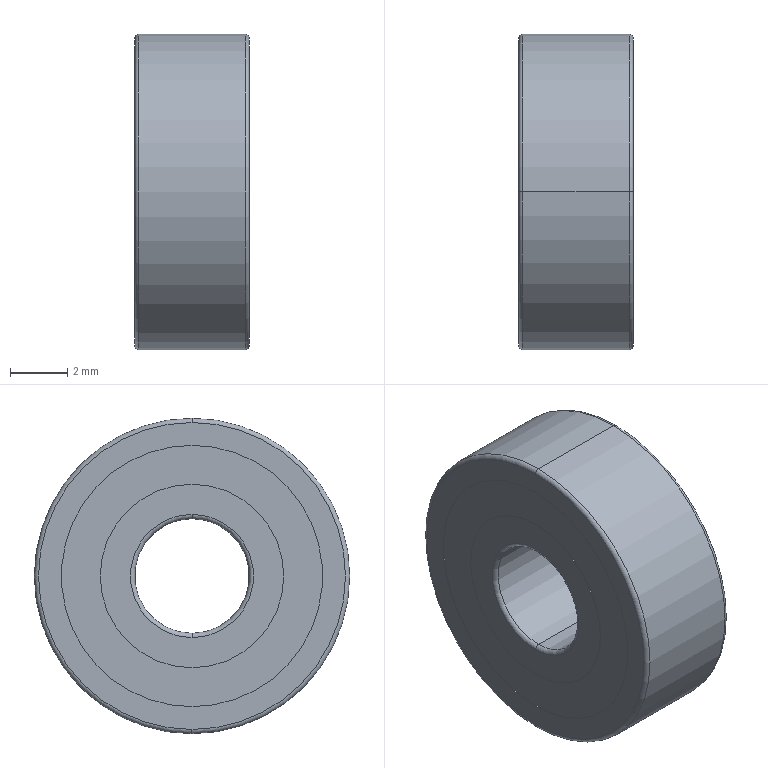Part | SolidWorks | features RefAxis 6, 3DProfileFeature 2, Revolution 1 | 1 solid | 26 faces | box 4 x 11 x 11 mm | volume 327.696 mm3 | cylinder 12 | torus 8 | plane 6 | commonest cylinder face diameters 6.4 x4 9.11 x4 4 x2 11 x2
STEP:
#1=CARTESIAN_POINT('',(3.85,0.,5.5));
#2=VERTEX_POINT('',#1);
#3=CARTESIAN_POINT('',(3.85,0.,-5.5));
#4=VERTEX_POINT('',#3);
#5=CARTESIAN_POINT('',(3.85,0.,0.));
#6=DIRECTION('',(-1.,0.,0.));
#7=DIRECTION('',(0.,0.,1.));
#8=AXIS2_PLACEMENT_3D('',#5,#6,#7);
#9=CIRCLE('',#8,5.5);
#10=EDGE_CURVE('',#2,#4,#9,.T.);
#11=ORIENTED_EDGE('',*,*,#10,.T.);
#12=CARTESIAN_POINT('',(0.15,0.,-5.5));
#13=VERTEX_POINT('',#12);
#14=CARTESIAN_POINT('',(3.85,0.,-5.5));
#15=DIRECTION('',(-1.,0.,0.));
#16=VECTOR('',#15,1000.);
#17=LINE('',#14,#16);
#18=EDGE_CURVE('',#4,#13,#17,.T.);
#19=ORIENTED_EDGE('',*,*,#18,.T.);
#20=CARTESIAN_POINT('',(0.15,0.,5.5));
#21=VERTEX_POINT('',#20);
#22=CARTESIAN_POINT('',(0.15,0.,0.));
#23=DIRECTION('',(-1.,0.,0.));
#24=DIRECTION('',(0.,0.,1.));
#25=AXIS2_PLACEMENT_3D('',#22,#23,#24);
#26=CIRCLE('',#25,5.5);
#27=EDGE_CURVE('',#21,#13,#26,.T.);
#28=ORIENTED_EDGE('',*,*,#27,.F.);
#29=CARTESIAN_POINT('',(3.85,0.,5.5));
#30=DIRECTION('',(-1.,0.,0.));
#31=VECTOR('',#30,1000.);
#32=LINE('',#29,#31);
#33=EDGE_CURVE('',#2,#21,#32,.T.);
#34=ORIENTED_EDGE('',*,*,#33,.F.);
#35=EDGE_LOOP('',(#11,#19,#28,#34));
#36=FACE_OUTER_BOUND('',#35,.T.);
#37=CARTESIAN_POINT('',(3.85,0.,0.));
#38=DIRECTION('',(-1.,0.,0.));
#39=DIRECTION('',(0.,0.,1.));
#40=AXIS2_PLACEMENT_3D('',#37,#38,#39);
#41=CYLINDRICAL_SURFACE('',#40,5.5);
#42=ADVANCED_FACE('',(#36),#41,.T.);
#43=CARTESIAN_POINT('',(4.,0.,5.35));
#44=VERTEX_POINT('',#43);
#45=CARTESIAN_POINT('',(4.,0.,-5.35));
#46=VERTEX_POINT('',#45);
#47=CARTESIAN_POINT('',(4.,0.,0.));
#48=DIRECTION('',(-1.,0.,0.));
#49=DIRECTION('',(0.,0.,1.));
#50=AXIS2_PLACEMENT_3D('',#47,#48,#49);
#51=CIRCLE('',#50,5.35);
#52=EDGE_CURVE('',#44,#46,#51,.T.);
#53=ORIENTED_EDGE('',*,*,#52,.T.);
#54=CARTESIAN_POINT('',(3.85,0.,-5.35));
#55=DIRECTION('',(0.,1.,0.));
#56=DIRECTION('',(0.,0.,1.));
#57=AXIS2_PLACEMENT_3D('',#54,#55,#56);
#58=CIRCLE('',#57,0.15);
#59=EDGE_CURVE('',#46,#4,#58,.T.);
#60=ORIENTED_EDGE('',*,*,#59,.T.);
#61=ORIENTED_EDGE('',*,*,#10,.F.);
#62=CARTESIAN_POINT('',(3.85,0.,5.35));
#63=DIRECTION('',(0.,-1.,0.));
#64=DIRECTION('',(0.,0.,-1.));
#65=AXIS2_PLACEMENT_3D('',#62,#63,#64);
#66=CIRCLE('',#65,0.15);
#67=EDGE_CURVE('',#44,#2,#66,.T.);
#68=ORIENTED_EDGE('',*,*,#67,.F.);
#69=EDGE_LOOP('',(#53,#60,#61,#68));
#70=FACE_OUTER_BOUND('',#69,.T.);
#71=CARTESIAN_POINT('',(3.85,0.,0.));
#72=DIRECTION('',(-1.,0.,0.));
#73=DIRECTION('',(0.,0.,1.));
#74=AXIS2_PLACEMENT_3D('',#71,#72,#73);
#75=TOROIDAL_SURFACE('',#74,5.35,0.15);
#76=ADVANCED_FACE('',(#70),#75,.T.);
#77=CARTESIAN_POINT('',(4.,0.,-4.555));
#78=VERTEX_POINT('',#77);
#79=CARTESIAN_POINT('',(4.,0.,4.555));
#80=VERTEX_POINT('',#79);
#81=CARTESIAN_POINT('',(4.,0.,0.));
#82=DIRECTION('',(-1.,0.,0.));
#83=DIRECTION('',(0.,0.,1.));
#84=AXIS2_PLACEMENT_3D('',#81,#82,#83);
#85=CIRCLE('',#84,4.555);
#86=EDGE_CURVE('',#78,#80,#85,.T.);
#87=ORIENTED_EDGE('',*,*,#86,.F.);
#88=CARTESIAN_POINT('',(3.974,0.,-4.555));
#89=VERTEX_POINT('',#88);
#90=CARTESIAN_POINT('',(3.85,0.,-4.555));
#91=DIRECTION('',(-1.,0.,0.));
#92=VECTOR('',#91,1000.);
#93=LINE('',#90,#92);
#94=EDGE_CURVE('',#78,#89,#93,.T.);
#95=ORIENTED_EDGE('',*,*,#94,.T.);
#96=CARTESIAN_POINT('',(3.974,0.,4.555));
#97=VERTEX_POINT('',#96);
#98=CARTESIAN_POINT('',(3.974,0.,0.));
#99=DIRECTION('',(-1.,0.,0.));
#100=DIRECTION('',(0.,0.,1.));
#101=AXIS2_PLACEMENT_3D('',#98,#99,#100);
#102=CIRCLE('',#101,4.555);
#103=EDGE_CURVE('',#89,#97,#102,.T.);
#104=ORIENTED_EDGE('',*,*,#103,.T.);
#105=CARTESIAN_POINT('',(3.85,0.,4.555));
#106=DIRECTION('',(-1.,0.,0.));
#107=VECTOR('',#106,1000.);
#108=LINE('',#105,#107);
#109=EDGE_CURVE('',#80,#97,#108,.T.);
#110=ORIENTED_EDGE('',*,*,#109,.F.);
#111=EDGE_LOOP('',(#87,#95,#104,#110));
#112=FACE_OUTER_BOUND('',#111,.T.);
#113=CARTESIAN_POINT('',(3.85,0.,0.));
#114=DIRECTION('',(-1.,0.,0.));
#115=DIRECTION('',(0.,0.,1.));
#116=AXIS2_PLACEMENT_3D('',#113,#114,#115);
#117=CYLINDRICAL_SURFACE('',#116,4.555);
#118=ADVANCED_FACE('',(#112),#117,.F.);
#119=CARTESIAN_POINT('',(4.,0.,3.2));
#120=VERTEX_POINT('',#119);
#121=CARTESIAN_POINT('',(4.,0.,-3.2));
#122=VERTEX_POINT('',#121);
#123=CARTESIAN_POINT('',(4.,0.,0.));
#124=DIRECTION('',(-1.,0.,0.));
#125=DIRECTION('',(0.,0.,1.));
#126=AXIS2_PLACEMENT_3D('',#123,#124,#125);
#127=CIRCLE('',#126,3.2);
#128=EDGE_CURVE('',#120,#122,#127,.T.);
#129=ORIENTED_EDGE('',*,*,#128,.T.);
#130=CARTESIAN_POINT('',(3.974,0.,-3.2));
#131=VERTEX_POINT('',#130);
#132=CARTESIAN_POINT('',(3.85,0.,-3.2));
#133=DIRECTION('',(-1.,0.,0.));
#134=VECTOR('',#133,1000.);
#135=LINE('',#132,#134);
#136=EDGE_CURVE('',#122,#131,#135,.T.);
#137=ORIENTED_EDGE('',*,*,#136,.T.);
#138=CARTESIAN_POINT('',(3.974,0.,3.2));
#139=VERTEX_POINT('',#138);
#140=CARTESIAN_POINT('',(3.974,0.,0.));
#141=DIRECTION('',(-1.,0.,0.));
#142=DIRECTION('',(0.,0.,1.));
#143=AXIS2_PLACEMENT_3D('',#140,#141,#142);
#144=CIRCLE('',#143,3.2);
#145=EDGE_CURVE('',#139,#131,#144,.T.);
#146=ORIENTED_EDGE('',*,*,#145,.F.);
#147=CARTESIAN_POINT('',(3.85,0.,3.2));
#148=DIRECTION('',(-1.,0.,0.));
#149=VECTOR('',#148,1000.);
#150=LINE('',#147,#149);
#151=EDGE_CURVE('',#120,#139,#150,.T.);
#152=ORIENTED_EDGE('',*,*,#151,.F.);
#153=EDGE_LOOP('',(#129,#137,#146,#152));
#154=FACE_OUTER_BOUND('',#153,.T.);
#155=CARTESIAN_POINT('',(3.85,0.,0.));
#156=DIRECTION('',(-1.,0.,0.));
#157=DIRECTION('',(0.,0.,1.));
#158=AXIS2_PLACEMENT_3D('',#155,#156,#157);
#159=CYLINDRICAL_SURFACE('',#158,3.2);
#160=ADVANCED_FACE('',(#154),#159,.T.);
#161=CARTESIAN_POINT('',(3.85,0.,2.));
#162=VERTEX_POINT('',#161);
#163=CARTESIAN_POINT('',(3.85,0.,-2.));
#164=VERTEX_POINT('',#163);
#165=CARTESIAN_POINT('',(3.85,0.,0.));
#166=DIRECTION('',(-1.,0.,0.));
#167=DIRECTION('',(0.,0.,1.));
#168=AXIS2_PLACEMENT_3D('',#165,#166,#167);
#169=CIRCLE('',#168,2.);
#170=EDGE_CURVE('',#162,#164,#169,.T.);
#171=ORIENTED_EDGE('',*,*,#170,.T.);
#172=CARTESIAN_POINT('',(4.,0.,-2.15));
#173=VERTEX_POINT('',#172);
#174=CARTESIAN_POINT('',(3.85,0.,-2.15));
#175=DIRECTION('',(0.,1.,0.));
#176=DIRECTION('',(0.,0.,1.));
#177=AXIS2_PLACEMENT_3D('',#174,#175,#176);
#178=CIRCLE('',#177,0.15);
#179=EDGE_CURVE('',#164,#173,#178,.T.);
#180=ORIENTED_EDGE('',*,*,#179,.T.);
#181=CARTESIAN_POINT('',(4.,0.,2.15));
#182=VERTEX_POINT('',#181);
#183=CARTESIAN_POINT('',(4.,0.,0.));
#184=DIRECTION('',(-1.,0.,0.));
#185=DIRECTION('',(0.,0.,1.));
#186=AXIS2_PLACEMENT_3D('',#183,#184,#185);
#187=CIRCLE('',#186,2.15);
#188=EDGE_CURVE('',#182,#173,#187,.T.);
#189=ORIENTED_EDGE('',*,*,#188,.F.);
#190=CARTESIAN_POINT('',(3.85,0.,2.15));
#191=DIRECTION('',(0.,-1.,0.));
#192=DIRECTION('',(0.,0.,-1.));
#193=AXIS2_PLACEMENT_3D('',#190,#191,#192);
#194=CIRCLE('',#193,0.15);
#195=EDGE_CURVE('',#162,#182,#194,.T.);
#196=ORIENTED_EDGE('',*,*,#195,.F.);
#197=EDGE_LOOP('',(#171,#180,#189,#196));
#198=FACE_OUTER_BOUND('',#197,.T.);
#199=CARTESIAN_POINT('',(3.85,0.,0.));
#200=DIRECTION('',(-1.,0.,0.));
#201=DIRECTION('',(0.,0.,1.));
#202=AXIS2_PLACEMENT_3D('',#199,#200,#201);
#203=TOROIDAL_SURFACE('',#202,2.15,0.15);
#204=ADVANCED_FACE('',(#198),#203,.T.);
#205=CARTESIAN_POINT('',(3.85,0.,0.));
#206=DIRECTION('',(-1.,0.,0.));
#207=DIRECTION('',(0.,0.,1.));
#208=AXIS2_PLACEMENT_3D('',#205,#206,#207);
#209=CIRCLE('',#208,2.);
#210=EDGE_CURVE('',#164,#162,#209,.T.);
#211=ORIENTED_EDGE('',*,*,#210,.F.);
#212=CARTESIAN_POINT('',(0.15,0.,-2.));
#213=VERTEX_POINT('',#212);
#214=CARTESIAN_POINT('',(3.85,0.,-2.));
#215=DIRECTION('',(-1.,0.,0.));
#216=VECTOR('',#215,1000.);
#217=LINE('',#214,#216);
#218=EDGE_CURVE('',#164,#213,#217,.T.);
#219=ORIENTED_EDGE('',*,*,#218,.T.);
#220=CARTESIAN_POINT('',(0.15,0.,2.));
#221=VERTEX_POINT('',#220);
#222=CARTESIAN_POINT('',(0.15,0.,0.));
#223=DIRECTION('',(-1.,0.,0.));
#224=DIRECTION('',(0.,0.,1.));
#225=AXIS2_PLACEMENT_3D('',#222,#223,#224);
#226=CIRCLE('',#225,2.);
#227=EDGE_CURVE('',#213,#221,#226,.T.);
#228=ORIENTED_EDGE('',*,*,#227,.T.);
#229=CARTESIAN_POINT('',(3.85,0.,2.));
#230=DIRECTION('',(-1.,0.,0.));
#231=VECTOR('',#230,1000.);
#232=LINE('',#229,#231);
#233=EDGE_CURVE('',#162,#221,#232,.T.);
#234=ORIENTED_EDGE('',*,*,#233,.F.);
#235=EDGE_LOOP('',(#211,#219,#228,#234));
#236=FACE_OUTER_BOUND('',#235,.T.);
#237=CARTESIAN_POINT('',(3.85,0.,0.));
#238=DIRECTION('',(-1.,0.,0.));
#239=DIRECTION('',(0.,0.,1.));
#240=AXIS2_PLACEMENT_3D('',#237,#238,#239);
#241=CYLINDRICAL_SURFACE('',#240,2.);
#242=ADVANCED_FACE('',(#236),#241,.F.);
#243=CARTESIAN_POINT('',(0.,0.,2.15));
#244=VERTEX_POINT('',#243);
#245=CARTESIAN_POINT('',(0.,0.,-2.15));
#246=VERTEX_POINT('',#245);
#247=CARTESIAN_POINT('',(0.,0.,0.));
#248=DIRECTION('',(-1.,0.,0.));
#249=DIRECTION('',(0.,0.,1.));
#250=AXIS2_PLACEMENT_3D('',#247,#248,#249);
#251=CIRCLE('',#250,2.15);
#252=EDGE_CURVE('',#244,#246,#251,.T.);
#253=ORIENTED_EDGE('',*,*,#252,.T.);
#254=CARTESIAN_POINT('',(0.15,0.,-2.15));
#255=DIRECTION('',(0.,1.,0.));
#256=DIRECTION('',(0.,0.,1.));
#257=AXIS2_PLACEMENT_3D('',#254,#255,#256);
#258=CIRCLE('',#257,0.15);
#259=EDGE_CURVE('',#246,#213,#258,.T.);
#260=ORIENTED_EDGE('',*,*,#259,.T.);
#261=CARTESIAN_POINT('',(0.15,0.,0.));
#262=DIRECTION('',(-1.,0.,0.));
#263=DIRECTION('',(0.,0.,1.));
#264=AXIS2_PLACEMENT_3D('',#261,#262,#263);
#265=CIRCLE('',#264,2.);
#266=EDGE_CURVE('',#221,#213,#265,.T.);
#267=ORIENTED_EDGE('',*,*,#266,.F.);
#268=CARTESIAN_POINT('',(0.15,0.,2.15));
#269=DIRECTION('',(0.,-1.,0.));
#270=DIRECTION('',(0.,0.,-1.));
#271=AXIS2_PLACEMENT_3D('',#268,#269,#270);
#272=CIRCLE('',#271,0.15);
#273=EDGE_CURVE('',#244,#221,#272,.T.);
#274=ORIENTED_EDGE('',*,*,#273,.F.);
#275=EDGE_LOOP('',(#253,#260,#267,#274));
#276=FACE_OUTER_BOUND('',#275,.T.);
#277=CARTESIAN_POINT('',(0.15,0.,0.));
#278=DIRECTION('',(-1.,0.,0.));
#279=DIRECTION('',(0.,0.,1.));
#280=AXIS2_PLACEMENT_3D('',#277,#278,#279);
#281=TOROIDAL_SURFACE('',#280,2.15,0.15);
#282=ADVANCED_FACE('',(#276),#281,.T.);
#283=CARTESIAN_POINT('',(0.026,0.,3.2));
#284=VERTEX_POINT('',#283);
#285=CARTESIAN_POINT('',(0.026,0.,-3.2));
#286=VERTEX_POINT('',#285);
#287=CARTESIAN_POINT('',(0.026,0.,0.));
#288=DIRECTION('',(-1.,0.,0.));
#289=DIRECTION('',(0.,0.,1.));
#290=AXIS2_PLACEMENT_3D('',#287,#288,#289);
#291=CIRCLE('',#290,3.2);
#292=EDGE_CURVE('',#284,#286,#291,.T.);
#293=ORIENTED_EDGE('',*,*,#292,.T.);
#294=CARTESIAN_POINT('',(0.,0.,-3.2));
#295=VERTEX_POINT('',#294);
#296=CARTESIAN_POINT('',(3.85,0.,-3.2));
#297=DIRECTION('',(-1.,0.,0.));
#298=VECTOR('',#297,1000.);
#299=LINE('',#296,#298);
#300=EDGE_CURVE('',#286,#295,#299,.T.);
#301=ORIENTED_EDGE('',*,*,#300,.T.);
#302=CARTESIAN_POINT('',(0.,0.,3.2));
#303=VERTEX_POINT('',#302);
#304=CARTESIAN_POINT('',(0.,0.,0.));
#305=DIRECTION('',(-1.,0.,0.));
#306=DIRECTION('',(0.,0.,1.));
#307=AXIS2_PLACEMENT_3D('',#304,#305,#306);
#308=CIRCLE('',#307,3.2);
#309=EDGE_CURVE('',#303,#295,#308,.T.);
#310=ORIENTED_EDGE('',*,*,#309,.F.);
#311=CARTESIAN_POINT('',(3.85,0.,3.2));
#312=DIRECTION('',(-1.,0.,0.));
#313=VECTOR('',#312,1000.);
#314=LINE('',#311,#313);
#315=EDGE_CURVE('',#284,#303,#314,.T.);
#316=ORIENTED_EDGE('',*,*,#315,.F.);
#317=EDGE_LOOP('',(#293,#301,#310,#316));
#318=FACE_OUTER_BOUND('',#317,.T.);
#319=CARTESIAN_POINT('',(3.85,0.,0.));
#320=DIRECTION('',(-1.,0.,0.));
#321=DIRECTION('',(0.,0.,1.));
#322=AXIS2_PLACEMENT_3D('',#319,#320,#321);
#323=CYLINDRICAL_SURFACE('',#322,3.2);
#324=ADVANCED_FACE('',(#318),#323,.T.);
#325=CARTESIAN_POINT('',(0.026,0.,-4.555));
#326=VERTEX_POINT('',#325);
#327=CARTESIAN_POINT('',(0.026,0.,4.555));
#328=VERTEX_POINT('',#327);
#329=CARTESIAN_POINT('',(0.026,0.,0.));
#330=DIRECTION('',(-1.,0.,0.));
#331=DIRECTION('',(0.,0.,1.));
#332=AXIS2_PLACEMENT_3D('',#329,#330,#331);
#333=CIRCLE('',#332,4.555);
#334=EDGE_CURVE('',#326,#328,#333,.T.);
#335=ORIENTED_EDGE('',*,*,#334,.F.);
#336=CARTESIAN_POINT('',(0.,0.,-4.555));
#337=VERTEX_POINT('',#336);
#338=CARTESIAN_POINT('',(3.85,0.,-4.555));
#339=DIRECTION('',(-1.,0.,0.));
#340=VECTOR('',#339,1000.);
#341=LINE('',#338,#340);
#342=EDGE_CURVE('',#326,#337,#341,.T.);
#343=ORIENTED_EDGE('',*,*,#342,.T.);
#344=CARTESIAN_POINT('',(0.,0.,4.555));
#345=VERTEX_POINT('',#344);
#346=CARTESIAN_POINT('',(0.,0.,0.));
#347=DIRECTION('',(-1.,0.,0.));
#348=DIRECTION('',(0.,0.,1.));
#349=AXIS2_PLACEMENT_3D('',#346,#347,#348);
#350=CIRCLE('',#349,4.555);
#351=EDGE_CURVE('',#337,#345,#350,.T.);
#352=ORIENTED_EDGE('',*,*,#351,.T.);
#353=CARTESIAN_POINT('',(3.85,0.,4.555));
#354=DIRECTION('',(-1.,0.,0.));
#355=VECTOR('',#354,1000.);
#356=LINE('',#353,#355);
#357=EDGE_CURVE('',#328,#345,#356,.T.);
#358=ORIENTED_EDGE('',*,*,#357,.F.);
#359=EDGE_LOOP('',(#335,#343,#352,#358));
#360=FACE_OUTER_BOUND('',#359,.T.);
#361=CARTESIAN_POINT('',(3.85,0.,0.));
#362=DIRECTION('',(-1.,0.,0.));
#363=DIRECTION('',(0.,0.,1.));
#364=AXIS2_PLACEMENT_3D('',#361,#362,#363);
#365=CYLINDRICAL_SURFACE('',#364,4.555);
#366=ADVANCED_FACE('',(#360),#365,.F.);
#367=ORIENTED_EDGE('',*,*,#27,.T.);
#368=CARTESIAN_POINT('',(0.,0.,-5.35));
#369=VERTEX_POINT('',#368);
#370=CARTESIAN_POINT('',(0.15,0.,-5.35));
#371=DIRECTION('',(0.,1.,0.));
#372=DIRECTION('',(0.,0.,1.));
#373=AXIS2_PLACEMENT_3D('',#370,#371,#372);
#374=CIRCLE('',#373,0.15);
#375=EDGE_CURVE('',#13,#369,#374,.T.);
#376=ORIENTED_EDGE('',*,*,#375,.T.);
#377=CARTESIAN_POINT('',(0.,0.,5.35));
#378=VERTEX_POINT('',#377);
#379=CARTESIAN_POINT('',(0.,0.,0.));
#380=DIRECTION('',(-1.,0.,0.));
#381=DIRECTION('',(0.,0.,1.));
#382=AXIS2_PLACEMENT_3D('',#379,#380,#381);
#383=CIRCLE('',#382,5.35);
#384=EDGE_CURVE('',#378,#369,#383,.T.);
#385=ORIENTED_EDGE('',*,*,#384,.F.);
#386=CARTESIAN_POINT('',(0.15,0.,5.35));
#387=DIRECTION('',(0.,-1.,0.));
#388=DIRECTION('',(0.,0.,-1.));
#389=AXIS2_PLACEMENT_3D('',#386,#387,#388);
#390=CIRCLE('',#389,0.15);
#391=EDGE_CURVE('',#21,#378,#390,.T.);
#392=ORIENTED_EDGE('',*,*,#391,.F.);
#393=EDGE_LOOP('',(#367,#376,#385,#392));
#394=FACE_OUTER_BOUND('',#393,.T.);
#395=CARTESIAN_POINT('',(0.15,0.,0.));
#396=DIRECTION('',(-1.,0.,0.));
#397=DIRECTION('',(0.,0.,1.));
#398=AXIS2_PLACEMENT_3D('',#395,#396,#397);
#399=TOROIDAL_SURFACE('',#398,5.35,0.15);
#400=ADVANCED_FACE('',(#394),#399,.T.);
#401=ORIENTED_EDGE('',*,*,#375,.F.);
#402=CARTESIAN_POINT('',(0.15,0.,0.));
#403=DIRECTION('',(-1.,0.,0.));
#404=DIRECTION('',(0.,0.,1.));
#405=AXIS2_PLACEMENT_3D('',#402,#403,#404);
#406=CIRCLE('',#405,5.5);
#407=EDGE_CURVE('',#13,#21,#406,.T.);
#408=ORIENTED_EDGE('',*,*,#407,.T.);
#409=ORIENTED_EDGE('',*,*,#391,.T.);
#410=CARTESIAN_POINT('',(0.,0.,0.));
#411=DIRECTION('',(-1.,0.,0.));
#412=DIRECTION('',(0.,0.,1.));
#413=AXIS2_PLACEMENT_3D('',#410,#411,#412);
#414=CIRCLE('',#413,5.35);
#415=EDGE_CURVE('',#369,#378,#414,.T.);
#416=ORIENTED_EDGE('',*,*,#415,.F.);
#417=EDGE_LOOP('',(#401,#408,#409,#416));
#418=FACE_OUTER_BOUND('',#417,.T.);
#419=CARTESIAN_POINT('',(0.15,0.,0.));
#420=DIRECTION('',(-1.,0.,0.));
#421=DIRECTION('',(0.,0.,1.));
#422=AXIS2_PLACEMENT_3D('',#419,#420,#421);
#423=TOROIDAL_SURFACE('',#422,5.35,0.15);
#424=ADVANCED_FACE('',(#418),#423,.T.);
#425=CARTESIAN_POINT('',(0.,0.,0.));
#426=DIRECTION('',(-1.,0.,0.));
#427=DIRECTION('',(0.,0.,1.));
#428=AXIS2_PLACEMENT_3D('',#425,#426,#427);
#429=CIRCLE('',#428,4.555);
#430=EDGE_CURVE('',#345,#337,#429,.T.);
#431=ORIENTED_EDGE('',*,*,#430,.F.);
#432=ORIENTED_EDGE('',*,*,#351,.F.);
#433=EDGE_LOOP('',(#431,#432));
#434=FACE_BOUND('',#433,.T.);
#435=ORIENTED_EDGE('',*,*,#384,.T.);
#436=ORIENTED_EDGE('',*,*,#415,.T.);
#437=EDGE_LOOP('',(#435,#436));
#438=FACE_OUTER_BOUND('',#437,.T.);
#439=CARTESIAN_POINT('',(0.,5.35,0.));
#440=DIRECTION('',(1.,0.,0.));
#441=DIRECTION('',(0.,0.,-1.));
#442=AXIS2_PLACEMENT_3D('',#439,#440,#441);
#443=PLANE('',#442);
#444=ADVANCED_FACE('',(#434,#438),#443,.F.);
#445=ORIENTED_EDGE('',*,*,#342,.F.);
#446=CARTESIAN_POINT('',(0.026,0.,0.));
#447=DIRECTION('',(-1.,0.,0.));
#448=DIRECTION('',(0.,0.,1.));
#449=AXIS2_PLACEMENT_3D('',#446,#447,#448);
#450=CIRCLE('',#449,4.555);
#451=EDGE_CURVE('',#328,#326,#450,.T.);
#452=ORIENTED_EDGE('',*,*,#451,.F.);
#453=ORIENTED_EDGE('',*,*,#357,.T.);
#454=ORIENTED_EDGE('',*,*,#430,.T.);
#455=EDGE_LOOP('',(#445,#452,#453,#454));
#456=FACE_OUTER_BOUND('',#455,.T.);
#457=CARTESIAN_POINT('',(3.85,0.,0.));
#458=DIRECTION('',(-1.,0.,0.));
#459=DIRECTION('',(0.,0.,1.));
#460=AXIS2_PLACEMENT_3D('',#457,#458,#459);
#461=CYLINDRICAL_SURFACE('',#460,4.555);
#462=ADVANCED_FACE('',(#456),#461,.F.);
#463=ORIENTED_EDGE('',*,*,#292,.F.);
#464=CARTESIAN_POINT('',(0.026,0.,0.));
#465=DIRECTION('',(-1.,0.,0.));
#466=DIRECTION('',(0.,0.,1.));
#467=AXIS2_PLACEMENT_3D('',#464,#465,#466);
#468=CIRCLE('',#467,3.2);
#469=EDGE_CURVE('',#286,#284,#468,.T.);
#470=ORIENTED_EDGE('',*,*,#469,.F.);
#471=EDGE_LOOP('',(#463,#470));
#472=FACE_BOUND('',#471,.T.);
#473=ORIENTED_EDGE('',*,*,#451,.T.);
#474=ORIENTED_EDGE('',*,*,#334,.T.);
#475=EDGE_LOOP('',(#473,#474));
#476=FACE_OUTER_BOUND('',#475,.T.);
#477=CARTESIAN_POINT('',(0.026,4.555,0.));
#478=DIRECTION('',(1.,0.,0.));
#479=DIRECTION('',(0.,0.,-1.));
#480=AXIS2_PLACEMENT_3D('',#477,#478,#479);
#481=PLANE('',#480);
#482=ADVANCED_FACE('',(#472,#476),#481,.F.);
#483=ORIENTED_EDGE('',*,*,#300,.F.);
#484=ORIENTED_EDGE('',*,*,#469,.T.);
#485=ORIENTED_EDGE('',*,*,#315,.T.);
#486=CARTESIAN_POINT('',(0.,0.,0.));
#487=DIRECTION('',(-1.,0.,0.));
#488=DIRECTION('',(0.,0.,1.));
#489=AXIS2_PLACEMENT_3D('',#486,#487,#488);
#490=CIRCLE('',#489,3.2);
#491=EDGE_CURVE('',#295,#303,#490,.T.);
#492=ORIENTED_EDGE('',*,*,#491,.F.);
#493=EDGE_LOOP('',(#483,#484,#485,#492));
#494=FACE_OUTER_BOUND('',#493,.T.);
#495=CARTESIAN_POINT('',(3.85,0.,0.));
#496=DIRECTION('',(-1.,0.,0.));
#497=DIRECTION('',(0.,0.,1.));
#498=AXIS2_PLACEMENT_3D('',#495,#496,#497);
#499=CYLINDRICAL_SURFACE('',#498,3.2);
#500=ADVANCED_FACE('',(#494),#499,.T.);
#501=ORIENTED_EDGE('',*,*,#252,.F.);
#502=CARTESIAN_POINT('',(0.,0.,0.));
#503=DIRECTION('',(-1.,0.,0.));
#504=DIRECTION('',(0.,0.,1.));
#505=AXIS2_PLACEMENT_3D('',#502,#503,#504);
#506=CIRCLE('',#505,2.15);
#507=EDGE_CURVE('',#246,#244,#506,.T.);
#508=ORIENTED_EDGE('',*,*,#507,.F.);
#509=EDGE_LOOP('',(#501,#508));
#510=FACE_BOUND('',#509,.T.);
#511=ORIENTED_EDGE('',*,*,#309,.T.);
#512=ORIENTED_EDGE('',*,*,#491,.T.);
#513=EDGE_LOOP('',(#511,#512));
#514=FACE_OUTER_BOUND('',#513,.T.);
#515=CARTESIAN_POINT('',(0.,3.2,0.));
#516=DIRECTION('',(1.,0.,0.));
#517=DIRECTION('',(0.,0.,-1.));
#518=AXIS2_PLACEMENT_3D('',#515,#516,#517);
#519=PLANE('',#518);
#520=ADVANCED_FACE('',(#510,#514),#519,.F.);
#521=ORIENTED_EDGE('',*,*,#259,.F.);
#522=ORIENTED_EDGE('',*,*,#507,.T.);
#523=ORIENTED_EDGE('',*,*,#273,.T.);
#524=ORIENTED_EDGE('',*,*,#227,.F.);
#525=EDGE_LOOP('',(#521,#522,#523,#524));
#526=FACE_OUTER_BOUND('',#525,.T.);
#527=CARTESIAN_POINT('',(0.15,0.,0.));
#528=DIRECTION('',(-1.,0.,0.));
#529=DIRECTION('',(0.,0.,1.));
#530=AXIS2_PLACEMENT_3D('',#527,#528,#529);
#531=TOROIDAL_SURFACE('',#530,2.15,0.15);
#532=ADVANCED_FACE('',(#526),#531,.T.);
#533=ORIENTED_EDGE('',*,*,#218,.F.);
#534=ORIENTED_EDGE('',*,*,#170,.F.);
#535=ORIENTED_EDGE('',*,*,#233,.T.);
#536=ORIENTED_EDGE('',*,*,#266,.T.);
#537=EDGE_LOOP('',(#533,#534,#535,#536));
#538=FACE_OUTER_BOUND('',#537,.T.);
#539=CARTESIAN_POINT('',(3.85,0.,0.));
#540=DIRECTION('',(-1.,0.,0.));
#541=DIRECTION('',(0.,0.,1.));
#542=AXIS2_PLACEMENT_3D('',#539,#540,#541);
#543=CYLINDRICAL_SURFACE('',#542,2.);
#544=ADVANCED_FACE('',(#538),#543,.F.);
#545=ORIENTED_EDGE('',*,*,#179,.F.);
#546=ORIENTED_EDGE('',*,*,#210,.T.);
#547=ORIENTED_EDGE('',*,*,#195,.T.);
#548=CARTESIAN_POINT('',(4.,0.,0.));
#549=DIRECTION('',(-1.,0.,0.));
#550=DIRECTION('',(0.,0.,1.));
#551=AXIS2_PLACEMENT_3D('',#548,#549,#550);
#552=CIRCLE('',#551,2.15);
#553=EDGE_CURVE('',#173,#182,#552,.T.);
#554=ORIENTED_EDGE('',*,*,#553,.F.);
#555=EDGE_LOOP('',(#545,#546,#547,#554));
#556=FACE_OUTER_BOUND('',#555,.T.);
#557=CARTESIAN_POINT('',(3.85,0.,0.));
#558=DIRECTION('',(-1.,0.,0.));
#559=DIRECTION('',(0.,0.,1.));
#560=AXIS2_PLACEMENT_3D('',#557,#558,#559);
#561=TOROIDAL_SURFACE('',#560,2.15,0.15);
#562=ADVANCED_FACE('',(#556),#561,.T.);
#563=ORIENTED_EDGE('',*,*,#128,.F.);
#564=CARTESIAN_POINT('',(4.,0.,0.));
#565=DIRECTION('',(-1.,0.,0.));
#566=DIRECTION('',(0.,0.,1.));
#567=AXIS2_PLACEMENT_3D('',#564,#565,#566);
#568=CIRCLE('',#567,3.2);
#569=EDGE_CURVE('',#122,#120,#568,.T.);
#570=ORIENTED_EDGE('',*,*,#569,.F.);
#571=EDGE_LOOP('',(#563,#570));
#572=FACE_OUTER_BOUND('',#571,.T.);
#573=ORIENTED_EDGE('',*,*,#188,.T.);
#574=ORIENTED_EDGE('',*,*,#553,.T.);
#575=EDGE_LOOP('',(#573,#574));
#576=FACE_BOUND('',#575,.T.);
#577=CARTESIAN_POINT('',(4.,2.15,0.));
#578=DIRECTION('',(-1.,0.,0.));
#579=DIRECTION('',(0.,0.,1.));
#580=AXIS2_PLACEMENT_3D('',#577,#578,#579);
#581=PLANE('',#580);
#582=ADVANCED_FACE('',(#572,#576),#581,.F.);
#583=ORIENTED_EDGE('',*,*,#136,.F.);
#584=ORIENTED_EDGE('',*,*,#569,.T.);
#585=ORIENTED_EDGE('',*,*,#151,.T.);
#586=CARTESIAN_POINT('',(3.974,0.,0.));
#587=DIRECTION('',(-1.,0.,0.));
#588=DIRECTION('',(0.,0.,1.));
#589=AXIS2_PLACEMENT_3D('',#586,#587,#588);
#590=CIRCLE('',#589,3.2);
#591=EDGE_CURVE('',#131,#139,#590,.T.);
#592=ORIENTED_EDGE('',*,*,#591,.F.);
#593=EDGE_LOOP('',(#583,#584,#585,#592));
#594=FACE_OUTER_BOUND('',#593,.T.);
#595=CARTESIAN_POINT('',(3.85,0.,0.));
#596=DIRECTION('',(-1.,0.,0.));
#597=DIRECTION('',(0.,0.,1.));
#598=AXIS2_PLACEMENT_3D('',#595,#596,#597);
#599=CYLINDRICAL_SURFACE('',#598,3.2);
#600=ADVANCED_FACE('',(#594),#599,.T.);
#601=CARTESIAN_POINT('',(3.974,0.,0.));
#602=DIRECTION('',(-1.,0.,0.));
#603=DIRECTION('',(0.,0.,1.));
#604=AXIS2_PLACEMENT_3D('',#601,#602,#603);
#605=CIRCLE('',#604,4.555);
#606=EDGE_CURVE('',#97,#89,#605,.T.);
#607=ORIENTED_EDGE('',*,*,#606,.F.);
#608=ORIENTED_EDGE('',*,*,#103,.F.);
#609=EDGE_LOOP('',(#607,#608));
#610=FACE_OUTER_BOUND('',#609,.T.);
#611=ORIENTED_EDGE('',*,*,#145,.T.);
#612=ORIENTED_EDGE('',*,*,#591,.T.);
#613=EDGE_LOOP('',(#611,#612));
#614=FACE_BOUND('',#613,.T.);
#615=CARTESIAN_POINT('',(3.974,3.2,0.));
#616=DIRECTION('',(-1.,0.,0.));
#617=DIRECTION('',(0.,0.,1.));
#618=AXIS2_PLACEMENT_3D('',#615,#616,#617);
#619=PLANE('',#618);
#620=ADVANCED_FACE('',(#610,#614),#619,.F.);
#621=ORIENTED_EDGE('',*,*,#94,.F.);
#622=CARTESIAN_POINT('',(4.,0.,0.));
#623=DIRECTION('',(-1.,0.,0.));
#624=DIRECTION('',(0.,0.,1.));
#625=AXIS2_PLACEMENT_3D('',#622,#623,#624);
#626=CIRCLE('',#625,4.555);
#627=EDGE_CURVE('',#80,#78,#626,.T.);
#628=ORIENTED_EDGE('',*,*,#627,.F.);
#629=ORIENTED_EDGE('',*,*,#109,.T.);
#630=ORIENTED_EDGE('',*,*,#606,.T.);
#631=EDGE_LOOP('',(#621,#628,#629,#630));
#632=FACE_OUTER_BOUND('',#631,.T.);
#633=CARTESIAN_POINT('',(3.85,0.,0.));
#634=DIRECTION('',(-1.,0.,0.));
#635=DIRECTION('',(0.,0.,1.));
#636=AXIS2_PLACEMENT_3D('',#633,#634,#635);
#637=CYLINDRICAL_SURFACE('',#636,4.555);
#638=ADVANCED_FACE('',(#632),#637,.F.);
#639=ORIENTED_EDGE('',*,*,#52,.F.);
#640=CARTESIAN_POINT('',(4.,0.,0.));
#641=DIRECTION('',(-1.,0.,0.));
#642=DIRECTION('',(0.,0.,1.));
#643=AXIS2_PLACEMENT_3D('',#640,#641,#642);
#644=CIRCLE('',#643,5.35);
#645=EDGE_CURVE('',#46,#44,#644,.T.);
#646=ORIENTED_EDGE('',*,*,#645,.F.);
#647=EDGE_LOOP('',(#639,#646));
#648=FACE_OUTER_BOUND('',#647,.T.);
#649=ORIENTED_EDGE('',*,*,#627,.T.);
#650=ORIENTED_EDGE('',*,*,#86,.T.);
#651=EDGE_LOOP('',(#649,#650));
#652=FACE_BOUND('',#651,.T.);
#653=CARTESIAN_POINT('',(4.,4.555,0.));
#654=DIRECTION('',(-1.,0.,0.));
#655=DIRECTION('',(0.,0.,1.));
#656=AXIS2_PLACEMENT_3D('',#653,#654,#655);
#657=PLANE('',#656);
#658=ADVANCED_FACE('',(#648,#652),#657,.F.);
#659=ORIENTED_EDGE('',*,*,#59,.F.);
#660=ORIENTED_EDGE('',*,*,#645,.T.);
#661=ORIENTED_EDGE('',*,*,#67,.T.);
#662=CARTESIAN_POINT('',(3.85,0.,0.));
#663=DIRECTION('',(-1.,0.,0.));
#664=DIRECTION('',(0.,0.,1.));
#665=AXIS2_PLACEMENT_3D('',#662,#663,#664);
#666=CIRCLE('',#665,5.5);
#667=EDGE_CURVE('',#4,#2,#666,.T.);
#668=ORIENTED_EDGE('',*,*,#667,.F.);
#669=EDGE_LOOP('',(#659,#660,#661,#668));
#670=FACE_OUTER_BOUND('',#669,.T.);
#671=CARTESIAN_POINT('',(3.85,0.,0.));
#672=DIRECTION('',(-1.,0.,0.));
#673=DIRECTION('',(0.,0.,1.));
#674=AXIS2_PLACEMENT_3D('',#671,#672,#673);
#675=TOROIDAL_SURFACE('',#674,5.35,0.15);
#676=ADVANCED_FACE('',(#670),#675,.T.);
#677=ORIENTED_EDGE('',*,*,#18,.F.);
#678=ORIENTED_EDGE('',*,*,#667,.T.);
#679=ORIENTED_EDGE('',*,*,#33,.T.);
#680=ORIENTED_EDGE('',*,*,#407,.F.);
#681=EDGE_LOOP('',(#677,#678,#679,#680));
#682=FACE_OUTER_BOUND('',#681,.T.);
#683=CARTESIAN_POINT('',(3.85,0.,0.));
#684=DIRECTION('',(-1.,0.,0.));
#685=DIRECTION('',(0.,0.,1.));
#686=AXIS2_PLACEMENT_3D('',#683,#684,#685);
#687=CYLINDRICAL_SURFACE('',#686,5.5);
#688=ADVANCED_FACE('',(#682),#687,.T.);
#689=CLOSED_SHELL('',(#42,#76,#118,#160,#204,#242,#282,#324,#366,#400,#424,#444,#462,#482,#500,#520,#532,#544,#562,#582,#600,#620,#638,#658,#676,#688));
#690=MANIFOLD_SOLID_BREP('',#689);
#691=CARTESIAN_POINT('',(0.,0.,0.));
#692=DIRECTION('',(0.,0.,1.));
#693=DIRECTION('',(1.,0.,0.));
#694=AXIS2_PLACEMENT_3D('',#691,#692,#693);
#695=(LENGTH_UNIT()NAMED_UNIT(*)SI_UNIT(.MILLI.,.METRE.));
#696=UNCERTAINTY_MEASURE_WITH_UNIT(LENGTH_MEASURE(0.00001),#695,'','');
#697=(NAMED_UNIT(*)PLANE_ANGLE_UNIT()SI_UNIT($,.RADIAN.));
#698=(NAMED_UNIT(*)SI_UNIT($,.STERADIAN.)SOLID_ANGLE_UNIT());
#699=(GEOMETRIC_REPRESENTATION_CONTEXT(3)GLOBAL_UNCERTAINTY_ASSIGNED_CONTEXT((#696))GLOBAL_UNIT_ASSIGNED_CONTEXT((#695,#697,#698))REPRESENTATION_CONTEXT('',''));
#700=ADVANCED_BREP_SHAPE_REPRESENTATION('',(#690,#694),#699);